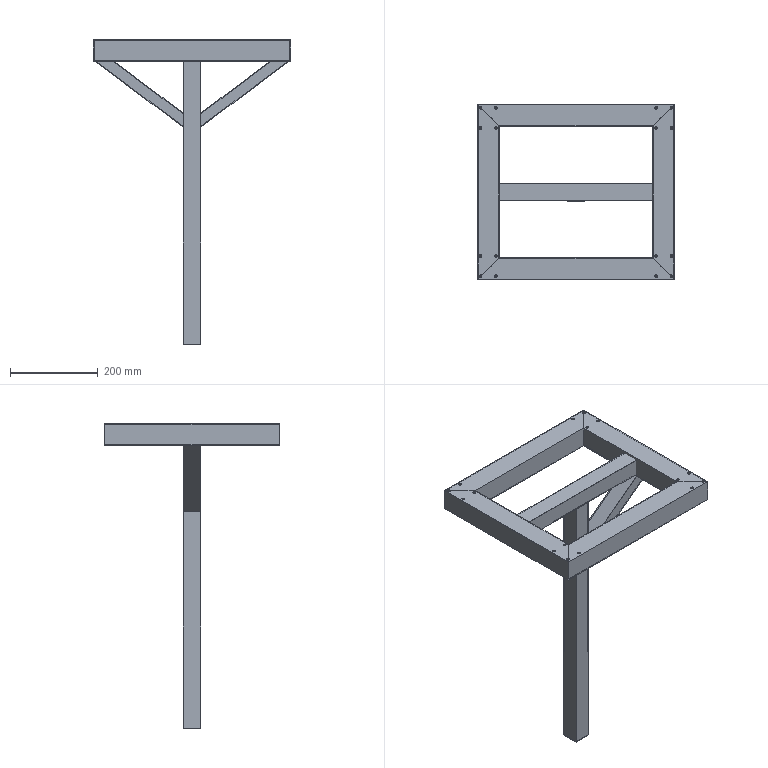Part | SolidWorks | features Shell 8, Gusset 2, ICE 2, WeldMemberFeat 2, HoleWzd 1, WeldmentFeature 1 | 8 solids | 152 faces | box 450 x 400 x 695 mm | volume 762729 mm3 | plane 80 | cone 36 | cylinder 36 | commonest cylinder face diameters 5 x36